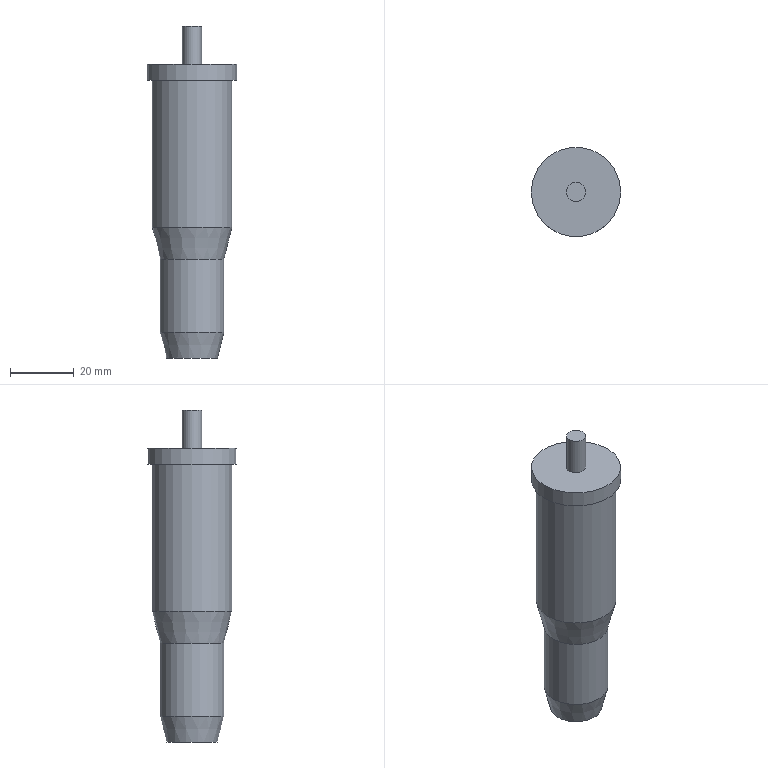Part | NX | features solid 2 | 1 solid | 10 faces | box 28 x 28 x 104 mm | volume 39260 mm3 | cylinder 4 | plane 4 | cone 2 | commonest cylinder face diameters 6 x1 20 x1 25 x1 28 x1
STEP:
#1=CARTESIAN_POINT('',(124.754,-309.832,34.));
#2=VERTEX_POINT('',#1);
#3=CARTESIAN_POINT('',(114.754,-309.832,34.));
#4=DIRECTION('',(0.,0.,1.));
#5=DIRECTION('',(1.,0.,0.));
#6=AXIS2_PLACEMENT_3D('',#3,#4,#5);
#7=CIRCLE('',#6,10.);
#8=EDGE_CURVE('',#2,#2,#7,.T.);
#9=ORIENTED_EDGE('',*,*,#8,.F.);
#10=EDGE_LOOP('',(#9));
#11=FACE_BOUND('',#10,.T.);
#12=CARTESIAN_POINT('',(124.754,-309.832,11.));
#13=VERTEX_POINT('',#12);
#14=CARTESIAN_POINT('',(114.754,-309.832,11.));
#15=DIRECTION('',(0.,0.,1.));
#16=DIRECTION('',(1.,0.,0.));
#17=AXIS2_PLACEMENT_3D('',#14,#15,#16);
#18=CIRCLE('',#17,10.);
#19=EDGE_CURVE('',#13,#13,#18,.T.);
#20=ORIENTED_EDGE('',*,*,#19,.T.);
#21=EDGE_LOOP('',(#20));
#22=FACE_BOUND('',#21,.T.);
#23=CARTESIAN_POINT('',(114.754,-309.832,13.));
#24=DIRECTION('',(0.,0.,1.));
#25=DIRECTION('',(1.,0.,0.));
#26=AXIS2_PLACEMENT_3D('',#23,#24,#25);
#27=CYLINDRICAL_SURFACE('',#26,10.);
#28=ADVANCED_FACE('',(#11,#22),#27,.T.);
#29=ORIENTED_EDGE('',*,*,#8,.T.);
#30=EDGE_LOOP('',(#29));
#31=FACE_BOUND('',#30,.T.);
#32=CARTESIAN_POINT('',(127.254,-309.832,44.));
#33=VERTEX_POINT('',#32);
#34=CARTESIAN_POINT('',(114.754,-309.832,44.));
#35=DIRECTION('',(0.,0.,1.));
#36=DIRECTION('',(1.,0.,0.));
#37=AXIS2_PLACEMENT_3D('',#34,#35,#36);
#38=CIRCLE('',#37,12.5);
#39=EDGE_CURVE('',#33,#33,#38,.T.);
#40=ORIENTED_EDGE('',*,*,#39,.F.);
#41=EDGE_LOOP('',(#40));
#42=FACE_BOUND('',#41,.T.);
#43=CARTESIAN_POINT('',(114.754,-309.832,34.));
#44=DIRECTION('',(0.,0.,1.));
#45=DIRECTION('',(1.,0.,0.));
#46=AXIS2_PLACEMENT_3D('',#43,#44,#45);
#47=CONICAL_SURFACE('',#46,10.,0.245);
#48=ADVANCED_FACE('',(#31,#42),#47,.T.);
#49=CARTESIAN_POINT('',(102.254,-309.832,90.));
#50=VERTEX_POINT('',#49);
#51=CARTESIAN_POINT('',(114.754,-309.832,90.));
#52=DIRECTION('',(0.,0.,-1.));
#53=DIRECTION('',(-1.,0.,0.));
#54=AXIS2_PLACEMENT_3D('',#51,#52,#53);
#55=CIRCLE('',#54,12.5);
#56=EDGE_CURVE('',#50,#50,#55,.F.);
#57=ORIENTED_EDGE('',*,*,#56,.F.);
#58=EDGE_LOOP('',(#57));
#59=FACE_BOUND('',#58,.T.);
#60=ORIENTED_EDGE('',*,*,#39,.T.);
#61=EDGE_LOOP('',(#60));
#62=FACE_BOUND('',#61,.T.);
#63=CARTESIAN_POINT('',(114.754,-309.832,44.));
#64=DIRECTION('',(0.,0.,1.));
#65=DIRECTION('',(1.,0.,0.));
#66=AXIS2_PLACEMENT_3D('',#63,#64,#65);
#67=CYLINDRICAL_SURFACE('',#66,12.5);
#68=ADVANCED_FACE('',(#59,#62),#67,.T.);
#69=CARTESIAN_POINT('',(117.754,-309.832,95.));
#70=VERTEX_POINT('',#69);
#71=CARTESIAN_POINT('',(114.754,-309.832,95.));
#72=DIRECTION('',(0.,0.,1.));
#73=DIRECTION('',(1.,0.,0.));
#74=AXIS2_PLACEMENT_3D('',#71,#72,#73);
#75=CIRCLE('',#74,3.);
#76=EDGE_CURVE('',#70,#70,#75,.T.);
#77=ORIENTED_EDGE('',*,*,#76,.F.);
#78=EDGE_LOOP('',(#77));
#79=FACE_BOUND('',#78,.T.);
#80=CARTESIAN_POINT('',(100.754,-309.832,95.));
#81=VERTEX_POINT('',#80);
#82=CARTESIAN_POINT('',(114.754,-309.832,95.));
#83=DIRECTION('',(0.,0.,-1.));
#84=DIRECTION('',(-1.,0.,0.));
#85=AXIS2_PLACEMENT_3D('',#82,#83,#84);
#86=CIRCLE('',#85,14.);
#87=EDGE_CURVE('',#81,#81,#86,.T.);
#88=ORIENTED_EDGE('',*,*,#87,.F.);
#89=EDGE_LOOP('',(#88));
#90=FACE_BOUND('',#89,.T.);
#91=CARTESIAN_POINT('',(114.754,-309.832,95.));
#92=DIRECTION('',(0.,0.,1.));
#93=DIRECTION('',(1.,0.,0.));
#94=AXIS2_PLACEMENT_3D('',#91,#92,#93);
#95=PLANE('',#94);
#96=ADVANCED_FACE('',(#79,#90),#95,.T.);
#97=ORIENTED_EDGE('',*,*,#56,.T.);
#98=EDGE_LOOP('',(#97));
#99=FACE_BOUND('',#98,.T.);
#100=CARTESIAN_POINT('',(128.754,-309.832,90.));
#101=VERTEX_POINT('',#100);
#102=CARTESIAN_POINT('',(114.754,-309.832,90.));
#103=DIRECTION('',(0.,0.,1.));
#104=DIRECTION('',(1.,0.,0.));
#105=AXIS2_PLACEMENT_3D('',#102,#103,#104);
#106=CIRCLE('',#105,14.);
#107=EDGE_CURVE('',#101,#101,#106,.T.);
#108=ORIENTED_EDGE('',*,*,#107,.F.);
#109=EDGE_LOOP('',(#108));
#110=FACE_BOUND('',#109,.T.);
#111=CARTESIAN_POINT('',(114.754,-309.832,90.));
#112=DIRECTION('',(0.,0.,-1.));
#113=DIRECTION('',(-1.,0.,0.));
#114=AXIS2_PLACEMENT_3D('',#111,#112,#113);
#115=PLANE('',#114);
#116=ADVANCED_FACE('',(#99,#110),#115,.T.);
#117=ORIENTED_EDGE('',*,*,#87,.T.);
#118=EDGE_LOOP('',(#117));
#119=FACE_BOUND('',#118,.T.);
#120=ORIENTED_EDGE('',*,*,#107,.T.);
#121=EDGE_LOOP('',(#120));
#122=FACE_BOUND('',#121,.T.);
#123=CARTESIAN_POINT('',(114.754,-309.832,90.));
#124=DIRECTION('',(0.,0.,1.));
#125=DIRECTION('',(1.,0.,0.));
#126=AXIS2_PLACEMENT_3D('',#123,#124,#125);
#127=CYLINDRICAL_SURFACE('',#126,14.);
#128=ADVANCED_FACE('',(#119,#122),#127,.T.);
#129=CARTESIAN_POINT('',(111.754,-309.832,107.));
#130=VERTEX_POINT('',#129);
#131=CARTESIAN_POINT('',(114.754,-309.832,107.));
#132=DIRECTION('',(0.,0.,-1.));
#133=DIRECTION('',(-1.,0.,0.));
#134=AXIS2_PLACEMENT_3D('',#131,#132,#133);
#135=CIRCLE('',#134,3.);
#136=EDGE_CURVE('',#130,#130,#135,.T.);
#137=ORIENTED_EDGE('',*,*,#136,.F.);
#138=EDGE_LOOP('',(#137));
#139=FACE_BOUND('',#138,.T.);
#140=CARTESIAN_POINT('',(114.754,-309.832,107.));
#141=DIRECTION('',(0.,0.,1.));
#142=DIRECTION('',(1.,0.,0.));
#143=AXIS2_PLACEMENT_3D('',#140,#141,#142);
#144=PLANE('',#143);
#145=ADVANCED_FACE('',(#139),#144,.T.);
#146=ORIENTED_EDGE('',*,*,#136,.T.);
#147=EDGE_LOOP('',(#146));
#148=FACE_BOUND('',#147,.T.);
#149=ORIENTED_EDGE('',*,*,#76,.T.);
#150=EDGE_LOOP('',(#149));
#151=FACE_BOUND('',#150,.T.);
#152=CARTESIAN_POINT('',(114.754,-309.832,95.));
#153=DIRECTION('',(0.,0.,1.));
#154=DIRECTION('',(1.,0.,0.));
#155=AXIS2_PLACEMENT_3D('',#152,#153,#154);
#156=CYLINDRICAL_SURFACE('',#155,3.);
#157=ADVANCED_FACE('',(#148,#151),#156,.T.);
#158=CARTESIAN_POINT('',(106.754,-309.832,3.));
#159=VERTEX_POINT('',#158);
#160=CARTESIAN_POINT('',(114.754,-309.832,3.));
#161=DIRECTION('',(0.,0.,-1.));
#162=DIRECTION('',(-1.,0.,0.));
#163=AXIS2_PLACEMENT_3D('',#160,#161,#162);
#164=CIRCLE('',#163,8.);
#165=EDGE_CURVE('',#159,#159,#164,.T.);
#166=ORIENTED_EDGE('',*,*,#165,.T.);
#167=EDGE_LOOP('',(#166));
#168=FACE_BOUND('',#167,.T.);
#169=CARTESIAN_POINT('',(114.754,-309.832,3.));
#170=DIRECTION('',(0.,0.,-1.));
#171=DIRECTION('',(-1.,0.,0.));
#172=AXIS2_PLACEMENT_3D('',#169,#170,#171);
#173=PLANE('',#172);
#174=ADVANCED_FACE('',(#168),#173,.T.);
#175=ORIENTED_EDGE('',*,*,#165,.F.);
#176=EDGE_LOOP('',(#175));
#177=FACE_BOUND('',#176,.T.);
#178=ORIENTED_EDGE('',*,*,#19,.F.);
#179=EDGE_LOOP('',(#178));
#180=FACE_BOUND('',#179,.T.);
#181=CARTESIAN_POINT('',(114.754,-309.832,11.));
#182=DIRECTION('',(0.,0.,1.));
#183=DIRECTION('',(1.,0.,0.));
#184=AXIS2_PLACEMENT_3D('',#181,#182,#183);
#185=CONICAL_SURFACE('',#184,10.,0.245);
#186=ADVANCED_FACE('',(#177,#180),#185,.T.);
#187=CLOSED_SHELL('',(#28,#48,#68,#96,#116,#128,#145,#157,#174,#186));
#188=MANIFOLD_SOLID_BREP('',#187);
#189=(LENGTH_UNIT()NAMED_UNIT(*)SI_UNIT(.MILLI.,.METRE.));
#190=UNCERTAINTY_MEASURE_WITH_UNIT(LENGTH_MEASURE(0.00001),#189,'','');
#191=(NAMED_UNIT(*)PLANE_ANGLE_UNIT()SI_UNIT($,.RADIAN.));
#192=(NAMED_UNIT(*)SI_UNIT($,.STERADIAN.)SOLID_ANGLE_UNIT());
#193=(GEOMETRIC_REPRESENTATION_CONTEXT(3)GLOBAL_UNCERTAINTY_ASSIGNED_CONTEXT((#190))GLOBAL_UNIT_ASSIGNED_CONTEXT((#189,#191,#192))REPRESENTATION_CONTEXT('',''));
#194=ADVANCED_BREP_SHAPE_REPRESENTATION('',(#188),#193);